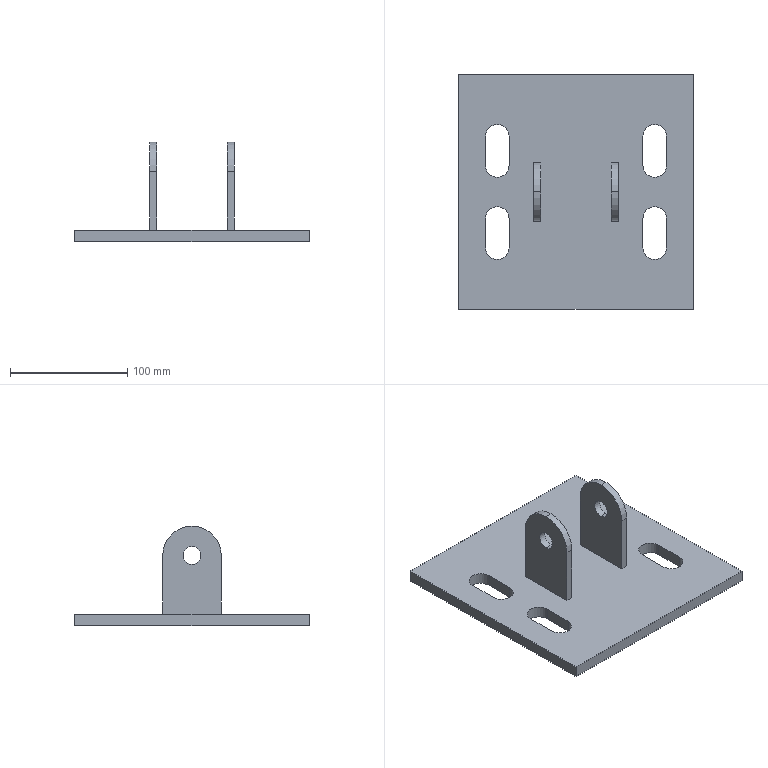Part | SolidWorks | features ICE 5, Extrusion 1 | 1 solid | 38 faces | box 200 x 200 x 85 mm | volume 407094 mm3 | plane 22 | cylinder 16 | commonest cylinder face diameters 20 x8 15 x4 50 x4
STEP:
#1=CARTESIAN_POINT('',(-30.,0.,47.5));
#2=VERTEX_POINT('',#1);
#3=CARTESIAN_POINT('',(-30.,0.,62.5));
#4=VERTEX_POINT('',#3);
#5=CARTESIAN_POINT('',(-30.,0.,55.));
#6=DIRECTION('',(-1.,0.,0.));
#7=DIRECTION('',(0.,0.,1.));
#8=AXIS2_PLACEMENT_3D('',#5,#6,#7);
#9=CIRCLE('',#8,7.5);
#10=EDGE_CURVE('',#2,#4,#9,.T.);
#11=ORIENTED_EDGE('',*,*,#10,.F.);
#12=CARTESIAN_POINT('',(-36.,0.,47.5));
#13=VERTEX_POINT('',#12);
#14=CARTESIAN_POINT('',(158.,0.,47.5));
#15=DIRECTION('',(-1.,0.,0.));
#16=VECTOR('',#15,1000.);
#17=LINE('',#14,#16);
#18=EDGE_CURVE('',#2,#13,#17,.T.);
#19=ORIENTED_EDGE('',*,*,#18,.T.);
#20=CARTESIAN_POINT('',(-36.,0.,62.5));
#21=VERTEX_POINT('',#20);
#22=CARTESIAN_POINT('',(-36.,0.,55.));
#23=DIRECTION('',(-1.,0.,0.));
#24=DIRECTION('',(0.,0.,1.));
#25=AXIS2_PLACEMENT_3D('',#22,#23,#24);
#26=CIRCLE('',#25,7.5);
#27=EDGE_CURVE('',#13,#21,#26,.T.);
#28=ORIENTED_EDGE('',*,*,#27,.T.);
#29=CARTESIAN_POINT('',(158.,0.,62.5));
#30=DIRECTION('',(-1.,0.,0.));
#31=VECTOR('',#30,1000.);
#32=LINE('',#29,#31);
#33=EDGE_CURVE('',#4,#21,#32,.T.);
#34=ORIENTED_EDGE('',*,*,#33,.F.);
#35=EDGE_LOOP('',(#11,#19,#28,#34));
#36=FACE_OUTER_BOUND('',#35,.T.);
#37=CARTESIAN_POINT('',(158.,0.,55.));
#38=DIRECTION('',(-1.,0.,0.));
#39=DIRECTION('',(0.,0.,1.));
#40=AXIS2_PLACEMENT_3D('',#37,#38,#39);
#41=CYLINDRICAL_SURFACE('',#40,7.5);
#42=ADVANCED_FACE('',(#36),#41,.F.);
#43=CARTESIAN_POINT('',(36.,0.,47.5));
#44=VERTEX_POINT('',#43);
#45=CARTESIAN_POINT('',(36.,0.,62.5));
#46=VERTEX_POINT('',#45);
#47=CARTESIAN_POINT('',(36.,0.,55.));
#48=DIRECTION('',(-1.,0.,0.));
#49=DIRECTION('',(0.,0.,1.));
#50=AXIS2_PLACEMENT_3D('',#47,#48,#49);
#51=CIRCLE('',#50,7.5);
#52=EDGE_CURVE('',#44,#46,#51,.T.);
#53=ORIENTED_EDGE('',*,*,#52,.F.);
#54=CARTESIAN_POINT('',(30.,0.,47.5));
#55=VERTEX_POINT('',#54);
#56=CARTESIAN_POINT('',(158.,0.,47.5));
#57=DIRECTION('',(-1.,0.,0.));
#58=VECTOR('',#57,1000.);
#59=LINE('',#56,#58);
#60=EDGE_CURVE('',#44,#55,#59,.T.);
#61=ORIENTED_EDGE('',*,*,#60,.T.);
#62=CARTESIAN_POINT('',(30.,0.,62.5));
#63=VERTEX_POINT('',#62);
#64=CARTESIAN_POINT('',(30.,0.,55.));
#65=DIRECTION('',(1.,0.,0.));
#66=DIRECTION('',(0.,0.,-1.));
#67=AXIS2_PLACEMENT_3D('',#64,#65,#66);
#68=CIRCLE('',#67,7.5);
#69=EDGE_CURVE('',#63,#55,#68,.T.);
#70=ORIENTED_EDGE('',*,*,#69,.F.);
#71=CARTESIAN_POINT('',(158.,0.,62.5));
#72=DIRECTION('',(-1.,0.,0.));
#73=VECTOR('',#72,1000.);
#74=LINE('',#71,#73);
#75=EDGE_CURVE('',#46,#63,#74,.T.);
#76=ORIENTED_EDGE('',*,*,#75,.F.);
#77=EDGE_LOOP('',(#53,#61,#70,#76));
#78=FACE_OUTER_BOUND('',#77,.T.);
#79=CARTESIAN_POINT('',(158.,0.,55.));
#80=DIRECTION('',(-1.,0.,0.));
#81=DIRECTION('',(0.,0.,1.));
#82=AXIS2_PLACEMENT_3D('',#79,#80,#81);
#83=CYLINDRICAL_SURFACE('',#82,7.5);
#84=ADVANCED_FACE('',(#78),#83,.F.);
#85=CARTESIAN_POINT('',(-30.,-25.,55.));
#86=VERTEX_POINT('',#85);
#87=CARTESIAN_POINT('',(-30.,0.,80.));
#88=VERTEX_POINT('',#87);
#89=CARTESIAN_POINT('',(-30.,0.,55.));
#90=DIRECTION('',(-1.,0.,0.));
#91=DIRECTION('',(0.,0.,1.));
#92=AXIS2_PLACEMENT_3D('',#89,#90,#91);
#93=CIRCLE('',#92,25.);
#94=EDGE_CURVE('',#86,#88,#93,.T.);
#95=ORIENTED_EDGE('',*,*,#94,.T.);
#96=CARTESIAN_POINT('',(-36.,0.,80.));
#97=VERTEX_POINT('',#96);
#98=CARTESIAN_POINT('',(-30.,0.,80.));
#99=DIRECTION('',(-1.,0.,0.));
#100=VECTOR('',#99,1000.);
#101=LINE('',#98,#100);
#102=EDGE_CURVE('',#88,#97,#101,.T.);
#103=ORIENTED_EDGE('',*,*,#102,.T.);
#104=CARTESIAN_POINT('',(-36.,-25.,55.));
#105=VERTEX_POINT('',#104);
#106=CARTESIAN_POINT('',(-36.,0.,55.));
#107=DIRECTION('',(-1.,0.,0.));
#108=DIRECTION('',(0.,0.,1.));
#109=AXIS2_PLACEMENT_3D('',#106,#107,#108);
#110=CIRCLE('',#109,25.);
#111=EDGE_CURVE('',#105,#97,#110,.T.);
#112=ORIENTED_EDGE('',*,*,#111,.F.);
#113=CARTESIAN_POINT('',(-36.,-25.,55.));
#114=DIRECTION('',(1.,0.,0.));
#115=VECTOR('',#114,1000.);
#116=LINE('',#113,#115);
#117=EDGE_CURVE('',#105,#86,#116,.T.);
#118=ORIENTED_EDGE('',*,*,#117,.T.);
#119=EDGE_LOOP('',(#95,#103,#112,#118));
#120=FACE_OUTER_BOUND('',#119,.T.);
#121=CARTESIAN_POINT('',(-30.,0.,55.));
#122=DIRECTION('',(-1.,0.,0.));
#123=DIRECTION('',(0.,0.,1.));
#124=AXIS2_PLACEMENT_3D('',#121,#122,#123);
#125=CYLINDRICAL_SURFACE('',#124,25.);
#126=ADVANCED_FACE('',(#120),#125,.T.);
#127=CARTESIAN_POINT('',(36.,-25.,55.));
#128=VERTEX_POINT('',#127);
#129=CARTESIAN_POINT('',(36.,0.,80.));
#130=VERTEX_POINT('',#129);
#131=CARTESIAN_POINT('',(36.,0.,55.));
#132=DIRECTION('',(-1.,0.,0.));
#133=DIRECTION('',(0.,0.,1.));
#134=AXIS2_PLACEMENT_3D('',#131,#132,#133);
#135=CIRCLE('',#134,25.);
#136=EDGE_CURVE('',#128,#130,#135,.T.);
#137=ORIENTED_EDGE('',*,*,#136,.T.);
#138=CARTESIAN_POINT('',(30.,0.,80.));
#139=VERTEX_POINT('',#138);
#140=CARTESIAN_POINT('',(36.,0.,80.));
#141=DIRECTION('',(-1.,0.,0.));
#142=VECTOR('',#141,1000.);
#143=LINE('',#140,#142);
#144=EDGE_CURVE('',#130,#139,#143,.T.);
#145=ORIENTED_EDGE('',*,*,#144,.T.);
#146=CARTESIAN_POINT('',(30.,-25.,55.));
#147=VERTEX_POINT('',#146);
#148=CARTESIAN_POINT('',(30.,0.,55.));
#149=DIRECTION('',(-1.,0.,0.));
#150=DIRECTION('',(0.,0.,1.));
#151=AXIS2_PLACEMENT_3D('',#148,#149,#150);
#152=CIRCLE('',#151,25.);
#153=EDGE_CURVE('',#147,#139,#152,.T.);
#154=ORIENTED_EDGE('',*,*,#153,.F.);
#155=CARTESIAN_POINT('',(36.,-25.,55.));
#156=DIRECTION('',(1.,0.,0.));
#157=VECTOR('',#156,1000.);
#158=LINE('',#155,#157);
#159=EDGE_CURVE('',#147,#128,#158,.T.);
#160=ORIENTED_EDGE('',*,*,#159,.T.);
#161=EDGE_LOOP('',(#137,#145,#154,#160));
#162=FACE_OUTER_BOUND('',#161,.T.);
#163=CARTESIAN_POINT('',(36.,0.,55.));
#164=DIRECTION('',(-1.,0.,0.));
#165=DIRECTION('',(0.,0.,1.));
#166=AXIS2_PLACEMENT_3D('',#163,#164,#165);
#167=CYLINDRICAL_SURFACE('',#166,25.);
#168=ADVANCED_FACE('',(#162),#167,.T.);
#169=CARTESIAN_POINT('',(57.064,47.5,5.));
#170=VERTEX_POINT('',#169);
#171=CARTESIAN_POINT('',(57.064,22.5,5.));
#172=VERTEX_POINT('',#171);
#173=CARTESIAN_POINT('',(57.064,47.5,5.));
#174=DIRECTION('',(0.,-1.,0.));
#175=VECTOR('',#174,1000.);
#176=LINE('',#173,#175);
#177=EDGE_CURVE('',#170,#172,#176,.T.);
#178=ORIENTED_EDGE('',*,*,#177,.F.);
#179=CARTESIAN_POINT('',(77.064,47.5,5.));
#180=VERTEX_POINT('',#179);
#181=CARTESIAN_POINT('',(67.064,47.5,5.));
#182=DIRECTION('',(0.,0.,1.));
#183=DIRECTION('',(-1.,0.,0.));
#184=AXIS2_PLACEMENT_3D('',#181,#182,#183);
#185=CIRCLE('',#184,10.);
#186=EDGE_CURVE('',#180,#170,#185,.T.);
#187=ORIENTED_EDGE('',*,*,#186,.F.);
#188=CARTESIAN_POINT('',(77.064,22.5,5.));
#189=VERTEX_POINT('',#188);
#190=CARTESIAN_POINT('',(77.064,47.5,5.));
#191=DIRECTION('',(0.,1.,0.));
#192=VECTOR('',#191,1000.);
#193=LINE('',#190,#192);
#194=EDGE_CURVE('',#189,#180,#193,.T.);
#195=ORIENTED_EDGE('',*,*,#194,.F.);
#196=CARTESIAN_POINT('',(67.064,22.5,5.));
#197=DIRECTION('',(0.,0.,1.));
#198=DIRECTION('',(-1.,0.,0.));
#199=AXIS2_PLACEMENT_3D('',#196,#197,#198);
#200=CIRCLE('',#199,10.);
#201=EDGE_CURVE('',#172,#189,#200,.T.);
#202=ORIENTED_EDGE('',*,*,#201,.F.);
#203=EDGE_LOOP('',(#178,#187,#195,#202));
#204=FACE_BOUND('',#203,.T.);
#205=CARTESIAN_POINT('',(57.064,-22.5,5.));
#206=VERTEX_POINT('',#205);
#207=CARTESIAN_POINT('',(57.064,-47.5,5.));
#208=VERTEX_POINT('',#207);
#209=CARTESIAN_POINT('',(57.064,-22.5,5.));
#210=DIRECTION('',(0.,-1.,0.));
#211=VECTOR('',#210,1000.);
#212=LINE('',#209,#211);
#213=EDGE_CURVE('',#206,#208,#212,.T.);
#214=ORIENTED_EDGE('',*,*,#213,.F.);
#215=CARTESIAN_POINT('',(77.064,-22.5,5.));
#216=VERTEX_POINT('',#215);
#217=CARTESIAN_POINT('',(67.064,-22.5,5.));
#218=DIRECTION('',(0.,0.,1.));
#219=DIRECTION('',(-1.,0.,0.));
#220=AXIS2_PLACEMENT_3D('',#217,#218,#219);
#221=CIRCLE('',#220,10.);
#222=EDGE_CURVE('',#216,#206,#221,.T.);
#223=ORIENTED_EDGE('',*,*,#222,.F.);
#224=CARTESIAN_POINT('',(77.064,-47.5,5.));
#225=VERTEX_POINT('',#224);
#226=CARTESIAN_POINT('',(77.064,-22.5,5.));
#227=DIRECTION('',(0.,1.,0.));
#228=VECTOR('',#227,1000.);
#229=LINE('',#226,#228);
#230=EDGE_CURVE('',#225,#216,#229,.T.);
#231=ORIENTED_EDGE('',*,*,#230,.F.);
#232=CARTESIAN_POINT('',(67.064,-47.5,5.));
#233=DIRECTION('',(0.,0.,1.));
#234=DIRECTION('',(-1.,0.,0.));
#235=AXIS2_PLACEMENT_3D('',#232,#233,#234);
#236=CIRCLE('',#235,10.);
#237=EDGE_CURVE('',#208,#225,#236,.T.);
#238=ORIENTED_EDGE('',*,*,#237,.F.);
#239=EDGE_LOOP('',(#214,#223,#231,#238));
#240=FACE_BOUND('',#239,.T.);
#241=CARTESIAN_POINT('',(-77.064,-22.5,5.));
#242=VERTEX_POINT('',#241);
#243=CARTESIAN_POINT('',(-77.064,-47.5,5.));
#244=VERTEX_POINT('',#243);
#245=CARTESIAN_POINT('',(-77.064,-22.5,5.));
#246=DIRECTION('',(0.,-1.,0.));
#247=VECTOR('',#246,1000.);
#248=LINE('',#245,#247);
#249=EDGE_CURVE('',#242,#244,#248,.T.);
#250=ORIENTED_EDGE('',*,*,#249,.F.);
#251=CARTESIAN_POINT('',(-57.064,-22.5,5.));
#252=VERTEX_POINT('',#251);
#253=CARTESIAN_POINT('',(-67.064,-22.5,5.));
#254=DIRECTION('',(0.,0.,1.));
#255=DIRECTION('',(1.,0.,0.));
#256=AXIS2_PLACEMENT_3D('',#253,#254,#255);
#257=CIRCLE('',#256,10.);
#258=EDGE_CURVE('',#252,#242,#257,.T.);
#259=ORIENTED_EDGE('',*,*,#258,.F.);
#260=CARTESIAN_POINT('',(-57.064,-47.5,5.));
#261=VERTEX_POINT('',#260);
#262=CARTESIAN_POINT('',(-57.064,-22.5,5.));
#263=DIRECTION('',(0.,1.,0.));
#264=VECTOR('',#263,1000.);
#265=LINE('',#262,#264);
#266=EDGE_CURVE('',#261,#252,#265,.T.);
#267=ORIENTED_EDGE('',*,*,#266,.F.);
#268=CARTESIAN_POINT('',(-67.064,-47.5,5.));
#269=DIRECTION('',(0.,0.,1.));
#270=DIRECTION('',(1.,0.,0.));
#271=AXIS2_PLACEMENT_3D('',#268,#269,#270);
#272=CIRCLE('',#271,10.);
#273=EDGE_CURVE('',#244,#261,#272,.T.);
#274=ORIENTED_EDGE('',*,*,#273,.F.);
#275=EDGE_LOOP('',(#250,#259,#267,#274));
#276=FACE_BOUND('',#275,.T.);
#277=CARTESIAN_POINT('',(-77.064,47.5,5.));
#278=VERTEX_POINT('',#277);
#279=CARTESIAN_POINT('',(-77.064,22.5,5.));
#280=VERTEX_POINT('',#279);
#281=CARTESIAN_POINT('',(-77.064,47.5,5.));
#282=DIRECTION('',(0.,-1.,0.));
#283=VECTOR('',#282,1000.);
#284=LINE('',#281,#283);
#285=EDGE_CURVE('',#278,#280,#284,.T.);
#286=ORIENTED_EDGE('',*,*,#285,.F.);
#287=CARTESIAN_POINT('',(-57.064,47.5,5.));
#288=VERTEX_POINT('',#287);
#289=CARTESIAN_POINT('',(-67.064,47.5,5.));
#290=DIRECTION('',(0.,0.,1.));
#291=DIRECTION('',(1.,0.,0.));
#292=AXIS2_PLACEMENT_3D('',#289,#290,#291);
#293=CIRCLE('',#292,10.);
#294=EDGE_CURVE('',#288,#278,#293,.T.);
#295=ORIENTED_EDGE('',*,*,#294,.F.);
#296=CARTESIAN_POINT('',(-57.064,22.5,5.));
#297=VERTEX_POINT('',#296);
#298=CARTESIAN_POINT('',(-57.064,47.5,5.));
#299=DIRECTION('',(0.,1.,0.));
#300=VECTOR('',#299,1000.);
#301=LINE('',#298,#300);
#302=EDGE_CURVE('',#297,#288,#301,.T.);
#303=ORIENTED_EDGE('',*,*,#302,.F.);
#304=CARTESIAN_POINT('',(-67.064,22.5,5.));
#305=DIRECTION('',(0.,0.,1.));
#306=DIRECTION('',(1.,0.,0.));
#307=AXIS2_PLACEMENT_3D('',#304,#305,#306);
#308=CIRCLE('',#307,10.);
#309=EDGE_CURVE('',#280,#297,#308,.T.);
#310=ORIENTED_EDGE('',*,*,#309,.F.);
#311=EDGE_LOOP('',(#286,#295,#303,#310));
#312=FACE_BOUND('',#311,.T.);
#313=CARTESIAN_POINT('',(-30.,-25.,5.));
#314=VERTEX_POINT('',#313);
#315=CARTESIAN_POINT('',(-30.,25.,5.));
#316=VERTEX_POINT('',#315);
#317=CARTESIAN_POINT('',(-30.,-25.,5.));
#318=DIRECTION('',(0.,1.,0.));
#319=VECTOR('',#318,1000.);
#320=LINE('',#317,#319);
#321=EDGE_CURVE('',#314,#316,#320,.T.);
#322=ORIENTED_EDGE('',*,*,#321,.F.);
#323=CARTESIAN_POINT('',(-36.,-25.,5.));
#324=VERTEX_POINT('',#323);
#325=CARTESIAN_POINT('',(-36.,-25.,5.));
#326=DIRECTION('',(1.,0.,0.));
#327=VECTOR('',#326,1000.);
#328=LINE('',#325,#327);
#329=EDGE_CURVE('',#324,#314,#328,.T.);
#330=ORIENTED_EDGE('',*,*,#329,.F.);
#331=CARTESIAN_POINT('',(-36.,25.,5.));
#332=VERTEX_POINT('',#331);
#333=CARTESIAN_POINT('',(-36.,-25.,5.));
#334=DIRECTION('',(0.,-1.,0.));
#335=VECTOR('',#334,1000.);
#336=LINE('',#333,#335);
#337=EDGE_CURVE('',#332,#324,#336,.T.);
#338=ORIENTED_EDGE('',*,*,#337,.F.);
#339=CARTESIAN_POINT('',(-36.,25.,5.));
#340=DIRECTION('',(-1.,0.,0.));
#341=VECTOR('',#340,1000.);
#342=LINE('',#339,#341);
#343=EDGE_CURVE('',#316,#332,#342,.T.);
#344=ORIENTED_EDGE('',*,*,#343,.F.);
#345=EDGE_LOOP('',(#322,#330,#338,#344));
#346=FACE_BOUND('',#345,.T.);
#347=CARTESIAN_POINT('',(-100.,100.,5.));
#348=VERTEX_POINT('',#347);
#349=CARTESIAN_POINT('',(-100.,-100.,5.));
#350=VERTEX_POINT('',#349);
#351=CARTESIAN_POINT('',(-100.,100.,5.));
#352=DIRECTION('',(0.,-1.,0.));
#353=VECTOR('',#352,1000.);
#354=LINE('',#351,#353);
#355=EDGE_CURVE('',#348,#350,#354,.T.);
#356=ORIENTED_EDGE('',*,*,#355,.T.);
#357=CARTESIAN_POINT('',(100.,-100.,5.));
#358=VERTEX_POINT('',#357);
#359=CARTESIAN_POINT('',(100.,-100.,5.));
#360=DIRECTION('',(1.,0.,0.));
#361=VECTOR('',#360,1000.);
#362=LINE('',#359,#361);
#363=EDGE_CURVE('',#350,#358,#362,.T.);
#364=ORIENTED_EDGE('',*,*,#363,.T.);
#365=CARTESIAN_POINT('',(100.,100.,5.));
#366=VERTEX_POINT('',#365);
#367=CARTESIAN_POINT('',(100.,100.,5.));
#368=DIRECTION('',(0.,1.,0.));
#369=VECTOR('',#368,1000.);
#370=LINE('',#367,#369);
#371=EDGE_CURVE('',#358,#366,#370,.T.);
#372=ORIENTED_EDGE('',*,*,#371,.T.);
#373=CARTESIAN_POINT('',(100.,100.,5.));
#374=DIRECTION('',(-1.,0.,0.));
#375=VECTOR('',#374,1000.);
#376=LINE('',#373,#375);
#377=EDGE_CURVE('',#366,#348,#376,.T.);
#378=ORIENTED_EDGE('',*,*,#377,.T.);
#379=EDGE_LOOP('',(#356,#364,#372,#378));
#380=FACE_OUTER_BOUND('',#379,.T.);
#381=CARTESIAN_POINT('',(36.,-25.,5.));
#382=VERTEX_POINT('',#381);
#383=CARTESIAN_POINT('',(36.,25.,5.));
#384=VERTEX_POINT('',#383);
#385=CARTESIAN_POINT('',(36.,-25.,5.));
#386=DIRECTION('',(0.,1.,0.));
#387=VECTOR('',#386,1000.);
#388=LINE('',#385,#387);
#389=EDGE_CURVE('',#382,#384,#388,.T.);
#390=ORIENTED_EDGE('',*,*,#389,.F.);
#391=CARTESIAN_POINT('',(30.,-25.,5.));
#392=VERTEX_POINT('',#391);
#393=CARTESIAN_POINT('',(36.,-25.,5.));
#394=DIRECTION('',(1.,0.,0.));
#395=VECTOR('',#394,1000.);
#396=LINE('',#393,#395);
#397=EDGE_CURVE('',#392,#382,#396,.T.);
#398=ORIENTED_EDGE('',*,*,#397,.F.);
#399=CARTESIAN_POINT('',(30.,25.,5.));
#400=VERTEX_POINT('',#399);
#401=CARTESIAN_POINT('',(30.,-25.,5.));
#402=DIRECTION('',(0.,-1.,0.));
#403=VECTOR('',#402,1000.);
#404=LINE('',#401,#403);
#405=EDGE_CURVE('',#400,#392,#404,.T.);
#406=ORIENTED_EDGE('',*,*,#405,.F.);
#407=CARTESIAN_POINT('',(36.,25.,5.));
#408=DIRECTION('',(-1.,0.,0.));
#409=VECTOR('',#408,1000.);
#410=LINE('',#407,#409);
#411=EDGE_CURVE('',#384,#400,#410,.T.);
#412=ORIENTED_EDGE('',*,*,#411,.F.);
#413=EDGE_LOOP('',(#390,#398,#406,#412));
#414=FACE_BOUND('',#413,.T.);
#415=CARTESIAN_POINT('',(0.,0.,5.));
#416=DIRECTION('',(0.,0.,-1.));
#417=DIRECTION('',(-1.,0.,0.));
#418=AXIS2_PLACEMENT_3D('',#415,#416,#417);
#419=PLANE('',#418);
#420=ADVANCED_FACE('',(#204,#240,#276,#312,#346,#380,#414),#419,.F.);
#421=CARTESIAN_POINT('',(-100.,-100.,-5.));
#422=VERTEX_POINT('',#421);
#423=CARTESIAN_POINT('',(-100.,-100.,-5.));
#424=DIRECTION('',(0.,0.,1.));
#425=VECTOR('',#424,1000.);
#426=LINE('',#423,#425);
#427=EDGE_CURVE('',#422,#350,#426,.T.);
#428=ORIENTED_EDGE('',*,*,#427,.T.);
#429=ORIENTED_EDGE('',*,*,#355,.F.);
#430=CARTESIAN_POINT('',(-100.,100.,-5.));
#431=VERTEX_POINT('',#430);
#432=CARTESIAN_POINT('',(-100.,100.,-5.));
#433=DIRECTION('',(0.,0.,1.));
#434=VECTOR('',#433,1000.);
#435=LINE('',#432,#434);
#436=EDGE_CURVE('',#431,#348,#435,.T.);
#437=ORIENTED_EDGE('',*,*,#436,.F.);
#438=CARTESIAN_POINT('',(-100.,100.,-5.));
#439=DIRECTION('',(0.,-1.,0.));
#440=VECTOR('',#439,1000.);
#441=LINE('',#438,#440);
#442=EDGE_CURVE('',#431,#422,#441,.T.);
#443=ORIENTED_EDGE('',*,*,#442,.T.);
#444=EDGE_LOOP('',(#428,#429,#437,#443));
#445=FACE_OUTER_BOUND('',#444,.T.);
#446=CARTESIAN_POINT('',(-100.,100.,-5.));
#447=DIRECTION('',(-1.,0.,0.));
#448=DIRECTION('',(0.,-1.,0.));
#449=AXIS2_PLACEMENT_3D('',#446,#447,#448);
#450=PLANE('',#449);
#451=ADVANCED_FACE('',(#445),#450,.T.);
#452=ORIENTED_EDGE('',*,*,#436,.T.);
#453=ORIENTED_EDGE('',*,*,#377,.F.);
#454=CARTESIAN_POINT('',(100.,100.,-5.));
#455=VERTEX_POINT('',#454);
#456=CARTESIAN_POINT('',(100.,100.,-5.));
#457=DIRECTION('',(0.,0.,1.));
#458=VECTOR('',#457,1000.);
#459=LINE('',#456,#458);
#460=EDGE_CURVE('',#455,#366,#459,.T.);
#461=ORIENTED_EDGE('',*,*,#460,.F.);
#462=CARTESIAN_POINT('',(100.,100.,-5.));
#463=DIRECTION('',(-1.,0.,0.));
#464=VECTOR('',#463,1000.);
#465=LINE('',#462,#464);
#466=EDGE_CURVE('',#455,#431,#465,.T.);
#467=ORIENTED_EDGE('',*,*,#466,.T.);
#468=EDGE_LOOP('',(#452,#453,#461,#467));
#469=FACE_OUTER_BOUND('',#468,.T.);
#470=CARTESIAN_POINT('',(100.,100.,-5.));
#471=DIRECTION('',(0.,1.,0.));
#472=DIRECTION('',(-1.,0.,0.));
#473=AXIS2_PLACEMENT_3D('',#470,#471,#472);
#474=PLANE('',#473);
#475=ADVANCED_FACE('',(#469),#474,.T.);
#476=ORIENTED_EDGE('',*,*,#460,.T.);
#477=ORIENTED_EDGE('',*,*,#371,.F.);
#478=CARTESIAN_POINT('',(100.,-100.,-5.));
#479=VERTEX_POINT('',#478);
#480=CARTESIAN_POINT('',(100.,-100.,-5.));
#481=DIRECTION('',(0.,0.,1.));
#482=VECTOR('',#481,1000.);
#483=LINE('',#480,#482);
#484=EDGE_CURVE('',#479,#358,#483,.T.);
#485=ORIENTED_EDGE('',*,*,#484,.F.);
#486=CARTESIAN_POINT('',(100.,100.,-5.));
#487=DIRECTION('',(0.,1.,0.));
#488=VECTOR('',#487,1000.);
#489=LINE('',#486,#488);
#490=EDGE_CURVE('',#479,#455,#489,.T.);
#491=ORIENTED_EDGE('',*,*,#490,.T.);
#492=EDGE_LOOP('',(#476,#477,#485,#491));
#493=FACE_OUTER_BOUND('',#492,.T.);
#494=CARTESIAN_POINT('',(100.,100.,-5.));
#495=DIRECTION('',(1.,0.,0.));
#496=DIRECTION('',(0.,1.,0.));
#497=AXIS2_PLACEMENT_3D('',#494,#495,#496);
#498=PLANE('',#497);
#499=ADVANCED_FACE('',(#493),#498,.T.);
#500=ORIENTED_EDGE('',*,*,#484,.T.);
#501=ORIENTED_EDGE('',*,*,#363,.F.);
#502=ORIENTED_EDGE('',*,*,#427,.F.);
#503=CARTESIAN_POINT('',(100.,-100.,-5.));
#504=DIRECTION('',(1.,0.,0.));
#505=VECTOR('',#504,1000.);
#506=LINE('',#503,#505);
#507=EDGE_CURVE('',#422,#479,#506,.T.);
#508=ORIENTED_EDGE('',*,*,#507,.T.);
#509=EDGE_LOOP('',(#500,#501,#502,#508));
#510=FACE_OUTER_BOUND('',#509,.T.);
#511=CARTESIAN_POINT('',(100.,-100.,-5.));
#512=DIRECTION('',(0.,-1.,0.));
#513=DIRECTION('',(1.,0.,0.));
#514=AXIS2_PLACEMENT_3D('',#511,#512,#513);
#515=PLANE('',#514);
#516=ADVANCED_FACE('',(#510),#515,.T.);
#517=CARTESIAN_POINT('',(77.064,47.5,-5.));
#518=VERTEX_POINT('',#517);
#519=CARTESIAN_POINT('',(57.064,47.5,-5.));
#520=VERTEX_POINT('',#519);
#521=CARTESIAN_POINT('',(67.064,47.5,-5.));
#522=DIRECTION('',(0.,0.,1.));
#523=DIRECTION('',(-1.,0.,0.));
#524=AXIS2_PLACEMENT_3D('',#521,#522,#523);
#525=CIRCLE('',#524,10.);
#526=EDGE_CURVE('',#518,#520,#525,.T.);
#527=ORIENTED_EDGE('',*,*,#526,.T.);
#528=CARTESIAN_POINT('',(57.064,22.5,-5.));
#529=VERTEX_POINT('',#528);
#530=CARTESIAN_POINT('',(57.064,47.5,-5.));
#531=DIRECTION('',(0.,-1.,0.));
#532=VECTOR('',#531,1000.);
#533=LINE('',#530,#532);
#534=EDGE_CURVE('',#520,#529,#533,.T.);
#535=ORIENTED_EDGE('',*,*,#534,.T.);
#536=CARTESIAN_POINT('',(77.064,22.5,-5.));
#537=VERTEX_POINT('',#536);
#538=CARTESIAN_POINT('',(67.064,22.5,-5.));
#539=DIRECTION('',(0.,0.,1.));
#540=DIRECTION('',(-1.,0.,0.));
#541=AXIS2_PLACEMENT_3D('',#538,#539,#540);
#542=CIRCLE('',#541,10.);
#543=EDGE_CURVE('',#529,#537,#542,.T.);
#544=ORIENTED_EDGE('',*,*,#543,.T.);
#545=CARTESIAN_POINT('',(77.064,47.5,-5.));
#546=DIRECTION('',(0.,1.,0.));
#547=VECTOR('',#546,1000.);
#548=LINE('',#545,#547);
#549=EDGE_CURVE('',#537,#518,#548,.T.);
#550=ORIENTED_EDGE('',*,*,#549,.T.);
#551=EDGE_LOOP('',(#527,#535,#544,#550));
#552=FACE_BOUND('',#551,.T.);
#553=CARTESIAN_POINT('',(77.064,-22.5,-5.));
#554=VERTEX_POINT('',#553);
#555=CARTESIAN_POINT('',(57.064,-22.5,-5.));
#556=VERTEX_POINT('',#555);
#557=CARTESIAN_POINT('',(67.064,-22.5,-5.));
#558=DIRECTION('',(0.,0.,1.));
#559=DIRECTION('',(-1.,0.,0.));
#560=AXIS2_PLACEMENT_3D('',#557,#558,#559);
#561=CIRCLE('',#560,10.);
#562=EDGE_CURVE('',#554,#556,#561,.T.);
#563=ORIENTED_EDGE('',*,*,#562,.T.);
#564=CARTESIAN_POINT('',(57.064,-47.5,-5.));
#565=VERTEX_POINT('',#564);
#566=CARTESIAN_POINT('',(57.064,-22.5,-5.));
#567=DIRECTION('',(0.,-1.,0.));
#568=VECTOR('',#567,1000.);
#569=LINE('',#566,#568);
#570=EDGE_CURVE('',#556,#565,#569,.T.);
#571=ORIENTED_EDGE('',*,*,#570,.T.);
#572=CARTESIAN_POINT('',(77.064,-47.5,-5.));
#573=VERTEX_POINT('',#572);
#574=CARTESIAN_POINT('',(67.064,-47.5,-5.));
#575=DIRECTION('',(0.,0.,1.));
#576=DIRECTION('',(-1.,0.,0.));
#577=AXIS2_PLACEMENT_3D('',#574,#575,#576);
#578=CIRCLE('',#577,10.);
#579=EDGE_CURVE('',#565,#573,#578,.T.);
#580=ORIENTED_EDGE('',*,*,#579,.T.);
#581=CARTESIAN_POINT('',(77.064,-22.5,-5.));
#582=DIRECTION('',(0.,1.,0.));
#583=VECTOR('',#582,1000.);
#584=LINE('',#581,#583);
#585=EDGE_CURVE('',#573,#554,#584,.T.);
#586=ORIENTED_EDGE('',*,*,#585,.T.);
#587=EDGE_LOOP('',(#563,#571,#580,#586));
#588=FACE_BOUND('',#587,.T.);
#589=CARTESIAN_POINT('',(-57.064,-22.5,-5.));
#590=VERTEX_POINT('',#589);
#591=CARTESIAN_POINT('',(-77.064,-22.5,-5.));
#592=VERTEX_POINT('',#591);
#593=CARTESIAN_POINT('',(-67.064,-22.5,-5.));
#594=DIRECTION('',(0.,0.,1.));
#595=DIRECTION('',(1.,0.,0.));
#596=AXIS2_PLACEMENT_3D('',#593,#594,#595);
#597=CIRCLE('',#596,10.);
#598=EDGE_CURVE('',#590,#592,#597,.T.);
#599=ORIENTED_EDGE('',*,*,#598,.T.);
#600=CARTESIAN_POINT('',(-77.064,-47.5,-5.));
#601=VERTEX_POINT('',#600);
#602=CARTESIAN_POINT('',(-77.064,-22.5,-5.));
#603=DIRECTION('',(0.,-1.,0.));
#604=VECTOR('',#603,1000.);
#605=LINE('',#602,#604);
#606=EDGE_CURVE('',#592,#601,#605,.T.);
#607=ORIENTED_EDGE('',*,*,#606,.T.);
#608=CARTESIAN_POINT('',(-57.064,-47.5,-5.));
#609=VERTEX_POINT('',#608);
#610=CARTESIAN_POINT('',(-67.064,-47.5,-5.));
#611=DIRECTION('',(0.,0.,1.));
#612=DIRECTION('',(1.,0.,0.));
#613=AXIS2_PLACEMENT_3D('',#610,#611,#612);
#614=CIRCLE('',#613,10.);
#615=EDGE_CURVE('',#601,#609,#614,.T.);
#616=ORIENTED_EDGE('',*,*,#615,.T.);
#617=CARTESIAN_POINT('',(-57.064,-22.5,-5.));
#618=DIRECTION('',(0.,1.,0.));
#619=VECTOR('',#618,1000.);
#620=LINE('',#617,#619);
#621=EDGE_CURVE('',#609,#590,#620,.T.);
#622=ORIENTED_EDGE('',*,*,#621,.T.);
#623=EDGE_LOOP('',(#599,#607,#616,#622));
#624=FACE_BOUND('',#623,.T.);
#625=CARTESIAN_POINT('',(-57.064,47.5,-5.));
#626=VERTEX_POINT('',#625);
#627=CARTESIAN_POINT('',(-77.064,47.5,-5.));
#628=VERTEX_POINT('',#627);
#629=CARTESIAN_POINT('',(-67.064,47.5,-5.));
#630=DIRECTION('',(0.,0.,1.));
#631=DIRECTION('',(1.,0.,0.));
#632=AXIS2_PLACEMENT_3D('',#629,#630,#631);
#633=CIRCLE('',#632,10.);
#634=EDGE_CURVE('',#626,#628,#633,.T.);
#635=ORIENTED_EDGE('',*,*,#634,.T.);
#636=CARTESIAN_POINT('',(-77.064,22.5,-5.));
#637=VERTEX_POINT('',#636);
#638=CARTESIAN_POINT('',(-77.064,47.5,-5.));
#639=DIRECTION('',(0.,-1.,0.));
#640=VECTOR('',#639,1000.);
#641=LINE('',#638,#640);
#642=EDGE_CURVE('',#628,#637,#641,.T.);
#643=ORIENTED_EDGE('',*,*,#642,.T.);
#644=CARTESIAN_POINT('',(-57.064,22.5,-5.));
#645=VERTEX_POINT('',#644);
#646=CARTESIAN_POINT('',(-67.064,22.5,-5.));
#647=DIRECTION('',(0.,0.,1.));
#648=DIRECTION('',(1.,0.,0.));
#649=AXIS2_PLACEMENT_3D('',#646,#647,#648);
#650=CIRCLE('',#649,10.);
#651=EDGE_CURVE('',#637,#645,#650,.T.);
#652=ORIENTED_EDGE('',*,*,#651,.T.);
#653=CARTESIAN_POINT('',(-57.064,47.5,-5.));
#654=DIRECTION('',(0.,1.,0.));
#655=VECTOR('',#654,1000.);
#656=LINE('',#653,#655);
#657=EDGE_CURVE('',#645,#626,#656,.T.);
#658=ORIENTED_EDGE('',*,*,#657,.T.);
#659=EDGE_LOOP('',(#635,#643,#652,#658));
#660=FACE_BOUND('',#659,.T.);
#661=ORIENTED_EDGE('',*,*,#442,.F.);
#662=ORIENTED_EDGE('',*,*,#466,.F.);
#663=ORIENTED_EDGE('',*,*,#490,.F.);
#664=ORIENTED_EDGE('',*,*,#507,.F.);
#665=EDGE_LOOP('',(#661,#662,#663,#664));
#666=FACE_OUTER_BOUND('',#665,.T.);
#667=CARTESIAN_POINT('',(0.,0.,-5.));
#668=DIRECTION('',(0.,0.,-1.));
#669=DIRECTION('',(-1.,0.,0.));
#670=AXIS2_PLACEMENT_3D('',#667,#668,#669);
#671=PLANE('',#670);
#672=ADVANCED_FACE('',(#552,#588,#624,#660,#666),#671,.T.);
#673=CARTESIAN_POINT('',(-30.,0.,55.));
#674=DIRECTION('',(-1.,0.,0.));
#675=DIRECTION('',(0.,0.,1.));
#676=AXIS2_PLACEMENT_3D('',#673,#674,#675);
#677=CIRCLE('',#676,7.5);
#678=EDGE_CURVE('',#4,#2,#677,.T.);
#679=ORIENTED_EDGE('',*,*,#678,.T.);
#680=ORIENTED_EDGE('',*,*,#10,.T.);
#681=EDGE_LOOP('',(#679,#680));
#682=FACE_BOUND('',#681,.T.);
#683=ORIENTED_EDGE('',*,*,#321,.T.);
#684=CARTESIAN_POINT('',(-30.,25.,55.));
#685=VERTEX_POINT('',#684);
#686=CARTESIAN_POINT('',(-30.,25.,55.));
#687=DIRECTION('',(0.,0.,-1.));
#688=VECTOR('',#687,1000.);
#689=LINE('',#686,#688);
#690=EDGE_CURVE('',#685,#316,#689,.T.);
#691=ORIENTED_EDGE('',*,*,#690,.F.);
#692=CARTESIAN_POINT('',(-30.,0.,55.));
#693=DIRECTION('',(-1.,0.,0.));
#694=DIRECTION('',(0.,0.,1.));
#695=AXIS2_PLACEMENT_3D('',#692,#693,#694);
#696=CIRCLE('',#695,25.);
#697=EDGE_CURVE('',#88,#685,#696,.T.);
#698=ORIENTED_EDGE('',*,*,#697,.F.);
#699=ORIENTED_EDGE('',*,*,#94,.F.);
#700=CARTESIAN_POINT('',(-30.,-25.,55.));
#701=DIRECTION('',(0.,0.,-1.));
#702=VECTOR('',#701,1000.);
#703=LINE('',#700,#702);
#704=EDGE_CURVE('',#86,#314,#703,.T.);
#705=ORIENTED_EDGE('',*,*,#704,.T.);
#706=EDGE_LOOP('',(#683,#691,#698,#699,#705));
#707=FACE_OUTER_BOUND('',#706,.T.);
#708=CARTESIAN_POINT('',(-30.,-25.,55.));
#709=DIRECTION('',(-1.,0.,0.));
#710=DIRECTION('',(0.,0.,1.));
#711=AXIS2_PLACEMENT_3D('',#708,#709,#710);
#712=PLANE('',#711);
#713=ADVANCED_FACE('',(#682,#707),#712,.F.);
#714=ORIENTED_EDGE('',*,*,#343,.T.);
#715=CARTESIAN_POINT('',(-36.,25.,55.));
#716=VERTEX_POINT('',#715);
#717=CARTESIAN_POINT('',(-36.,25.,55.));
#718=DIRECTION('',(0.,0.,-1.));
#719=VECTOR('',#718,1000.);
#720=LINE('',#717,#719);
#721=EDGE_CURVE('',#716,#332,#720,.T.);
#722=ORIENTED_EDGE('',*,*,#721,.F.);
#723=CARTESIAN_POINT('',(-36.,25.,55.));
#724=DIRECTION('',(-1.,0.,0.));
#725=VECTOR('',#724,1000.);
#726=LINE('',#723,#725);
#727=EDGE_CURVE('',#685,#716,#726,.T.);
#728=ORIENTED_EDGE('',*,*,#727,.F.);
#729=ORIENTED_EDGE('',*,*,#690,.T.);
#730=EDGE_LOOP('',(#714,#722,#728,#729));
#731=FACE_OUTER_BOUND('',#730,.T.);
#732=CARTESIAN_POINT('',(-36.,25.,55.));
#733=DIRECTION('',(0.,-1.,0.));
#734=DIRECTION('',(0.,0.,-1.));
#735=AXIS2_PLACEMENT_3D('',#732,#733,#734);
#736=PLANE('',#735);
#737=ADVANCED_FACE('',(#731),#736,.F.);
#738=CARTESIAN_POINT('',(-36.,0.,55.));
#739=DIRECTION('',(-1.,0.,0.));
#740=DIRECTION('',(0.,0.,1.));
#741=AXIS2_PLACEMENT_3D('',#738,#739,#740);
#742=CIRCLE('',#741,7.5);
#743=EDGE_CURVE('',#21,#13,#742,.T.);
#744=ORIENTED_EDGE('',*,*,#743,.F.);
#745=ORIENTED_EDGE('',*,*,#27,.F.);
#746=EDGE_LOOP('',(#744,#745));
#747=FACE_BOUND('',#746,.T.);
#748=ORIENTED_EDGE('',*,*,#337,.T.);
#749=CARTESIAN_POINT('',(-36.,-25.,55.));
#750=DIRECTION('',(0.,0.,-1.));
#751=VECTOR('',#750,1000.);
#752=LINE('',#749,#751);
#753=EDGE_CURVE('',#105,#324,#752,.T.);
#754=ORIENTED_EDGE('',*,*,#753,.F.);
#755=ORIENTED_EDGE('',*,*,#111,.T.);
#756=CARTESIAN_POINT('',(-36.,0.,55.));
#757=DIRECTION('',(-1.,0.,0.));
#758=DIRECTION('',(0.,0.,1.));
#759=AXIS2_PLACEMENT_3D('',#756,#757,#758);
#760=CIRCLE('',#759,25.);
#761=EDGE_CURVE('',#97,#716,#760,.T.);
#762=ORIENTED_EDGE('',*,*,#761,.T.);
#763=ORIENTED_EDGE('',*,*,#721,.T.);
#764=EDGE_LOOP('',(#748,#754,#755,#762,#763));
#765=FACE_OUTER_BOUND('',#764,.T.);
#766=CARTESIAN_POINT('',(-36.,-25.,55.));
#767=DIRECTION('',(1.,0.,0.));
#768=DIRECTION('',(0.,0.,-1.));
#769=AXIS2_PLACEMENT_3D('',#766,#767,#768);
#770=PLANE('',#769);
#771=ADVANCED_FACE('',(#747,#765),#770,.F.);
#772=ORIENTED_EDGE('',*,*,#329,.T.);
#773=ORIENTED_EDGE('',*,*,#704,.F.);
#774=ORIENTED_EDGE('',*,*,#117,.F.);
#775=ORIENTED_EDGE('',*,*,#753,.T.);
#776=EDGE_LOOP('',(#772,#773,#774,#775));
#777=FACE_OUTER_BOUND('',#776,.T.);
#778=CARTESIAN_POINT('',(-36.,-25.,55.));
#779=DIRECTION('',(0.,1.,0.));
#780=DIRECTION('',(0.,0.,1.));
#781=AXIS2_PLACEMENT_3D('',#778,#779,#780);
#782=PLANE('',#781);
#783=ADVANCED_FACE('',(#777),#782,.F.);
#784=CARTESIAN_POINT('',(36.,0.,55.));
#785=DIRECTION('',(-1.,0.,0.));
#786=DIRECTION('',(0.,0.,1.));
#787=AXIS2_PLACEMENT_3D('',#784,#785,#786);
#788=CIRCLE('',#787,7.5);
#789=EDGE_CURVE('',#46,#44,#788,.T.);
#790=ORIENTED_EDGE('',*,*,#789,.T.);
#791=ORIENTED_EDGE('',*,*,#52,.T.);
#792=EDGE_LOOP('',(#790,#791));
#793=FACE_BOUND('',#792,.T.);
#794=ORIENTED_EDGE('',*,*,#389,.T.);
#795=CARTESIAN_POINT('',(36.,25.,55.));
#796=VERTEX_POINT('',#795);
#797=CARTESIAN_POINT('',(36.,25.,55.));
#798=DIRECTION('',(0.,0.,-1.));
#799=VECTOR('',#798,1000.);
#800=LINE('',#797,#799);
#801=EDGE_CURVE('',#796,#384,#800,.T.);
#802=ORIENTED_EDGE('',*,*,#801,.F.);
#803=CARTESIAN_POINT('',(36.,0.,55.));
#804=DIRECTION('',(-1.,0.,0.));
#805=DIRECTION('',(0.,0.,1.));
#806=AXIS2_PLACEMENT_3D('',#803,#804,#805);
#807=CIRCLE('',#806,25.);
#808=EDGE_CURVE('',#130,#796,#807,.T.);
#809=ORIENTED_EDGE('',*,*,#808,.F.);
#810=ORIENTED_EDGE('',*,*,#136,.F.);
#811=CARTESIAN_POINT('',(36.,-25.,55.));
#812=DIRECTION('',(0.,0.,-1.));
#813=VECTOR('',#812,1000.);
#814=LINE('',#811,#813);
#815=EDGE_CURVE('',#128,#382,#814,.T.);
#816=ORIENTED_EDGE('',*,*,#815,.T.);
#817=EDGE_LOOP('',(#794,#802,#809,#810,#816));
#818=FACE_OUTER_BOUND('',#817,.T.);
#819=CARTESIAN_POINT('',(36.,-25.,55.));
#820=DIRECTION('',(-1.,0.,0.));
#821=DIRECTION('',(0.,0.,1.));
#822=AXIS2_PLACEMENT_3D('',#819,#820,#821);
#823=PLANE('',#822);
#824=ADVANCED_FACE('',(#793,#818),#823,.F.);
#825=ORIENTED_EDGE('',*,*,#411,.T.);
#826=CARTESIAN_POINT('',(30.,25.,55.));
#827=VERTEX_POINT('',#826);
#828=CARTESIAN_POINT('',(30.,25.,55.));
#829=DIRECTION('',(0.,0.,-1.));
#830=VECTOR('',#829,1000.);
#831=LINE('',#828,#830);
#832=EDGE_CURVE('',#827,#400,#831,.T.);
#833=ORIENTED_EDGE('',*,*,#832,.F.);
#834=CARTESIAN_POINT('',(36.,25.,55.));
#835=DIRECTION('',(-1.,0.,0.));
#836=VECTOR('',#835,1000.);
#837=LINE('',#834,#836);
#838=EDGE_CURVE('',#796,#827,#837,.T.);
#839=ORIENTED_EDGE('',*,*,#838,.F.);
#840=ORIENTED_EDGE('',*,*,#801,.T.);
#841=EDGE_LOOP('',(#825,#833,#839,#840));
#842=FACE_OUTER_BOUND('',#841,.T.);
#843=CARTESIAN_POINT('',(36.,25.,55.));
#844=DIRECTION('',(0.,-1.,0.));
#845=DIRECTION('',(0.,0.,-1.));
#846=AXIS2_PLACEMENT_3D('',#843,#844,#845);
#847=PLANE('',#846);
#848=ADVANCED_FACE('',(#842),#847,.F.);
#849=ORIENTED_EDGE('',*,*,#69,.T.);
#850=CARTESIAN_POINT('',(30.,0.,55.));
#851=DIRECTION('',(1.,0.,0.));
#852=DIRECTION('',(0.,0.,-1.));
#853=AXIS2_PLACEMENT_3D('',#850,#851,#852);
#854=CIRCLE('',#853,7.5);
#855=EDGE_CURVE('',#55,#63,#854,.T.);
#856=ORIENTED_EDGE('',*,*,#855,.T.);
#857=EDGE_LOOP('',(#849,#856));
#858=FACE_BOUND('',#857,.T.);
#859=ORIENTED_EDGE('',*,*,#405,.T.);
#860=CARTESIAN_POINT('',(30.,-25.,55.));
#861=DIRECTION('',(0.,0.,-1.));
#862=VECTOR('',#861,1000.);
#863=LINE('',#860,#862);
#864=EDGE_CURVE('',#147,#392,#863,.T.);
#865=ORIENTED_EDGE('',*,*,#864,.F.);
#866=ORIENTED_EDGE('',*,*,#153,.T.);
#867=CARTESIAN_POINT('',(30.,0.,55.));
#868=DIRECTION('',(-1.,0.,0.));
#869=DIRECTION('',(0.,0.,1.));
#870=AXIS2_PLACEMENT_3D('',#867,#868,#869);
#871=CIRCLE('',#870,25.);
#872=EDGE_CURVE('',#139,#827,#871,.T.);
#873=ORIENTED_EDGE('',*,*,#872,.T.);
#874=ORIENTED_EDGE('',*,*,#832,.T.);
#875=EDGE_LOOP('',(#859,#865,#866,#873,#874));
#876=FACE_OUTER_BOUND('',#875,.T.);
#877=CARTESIAN_POINT('',(30.,-25.,55.));
#878=DIRECTION('',(1.,0.,0.));
#879=DIRECTION('',(0.,0.,-1.));
#880=AXIS2_PLACEMENT_3D('',#877,#878,#879);
#881=PLANE('',#880);
#882=ADVANCED_FACE('',(#858,#876),#881,.F.);
#883=ORIENTED_EDGE('',*,*,#397,.T.);
#884=ORIENTED_EDGE('',*,*,#815,.F.);
#885=ORIENTED_EDGE('',*,*,#159,.F.);
#886=ORIENTED_EDGE('',*,*,#864,.T.);
#887=EDGE_LOOP('',(#883,#884,#885,#886));
#888=FACE_OUTER_BOUND('',#887,.T.);
#889=CARTESIAN_POINT('',(36.,-25.,55.));
#890=DIRECTION('',(0.,1.,0.));
#891=DIRECTION('',(0.,0.,1.));
#892=AXIS2_PLACEMENT_3D('',#889,#890,#891);
#893=PLANE('',#892);
#894=ADVANCED_FACE('',(#888),#893,.F.);
#895=ORIENTED_EDGE('',*,*,#144,.F.);
#896=ORIENTED_EDGE('',*,*,#808,.T.);
#897=ORIENTED_EDGE('',*,*,#838,.T.);
#898=ORIENTED_EDGE('',*,*,#872,.F.);
#899=EDGE_LOOP('',(#895,#896,#897,#898));
#900=FACE_OUTER_BOUND('',#899,.T.);
#901=CARTESIAN_POINT('',(36.,0.,55.));
#902=DIRECTION('',(-1.,0.,0.));
#903=DIRECTION('',(0.,0.,1.));
#904=AXIS2_PLACEMENT_3D('',#901,#902,#903);
#905=CYLINDRICAL_SURFACE('',#904,25.);
#906=ADVANCED_FACE('',(#900),#905,.T.);
#907=ORIENTED_EDGE('',*,*,#102,.F.);
#908=ORIENTED_EDGE('',*,*,#697,.T.);
#909=ORIENTED_EDGE('',*,*,#727,.T.);
#910=ORIENTED_EDGE('',*,*,#761,.F.);
#911=EDGE_LOOP('',(#907,#908,#909,#910));
#912=FACE_OUTER_BOUND('',#911,.T.);
#913=CARTESIAN_POINT('',(-30.,0.,55.));
#914=DIRECTION('',(-1.,0.,0.));
#915=DIRECTION('',(0.,0.,1.));
#916=AXIS2_PLACEMENT_3D('',#913,#914,#915);
#917=CYLINDRICAL_SURFACE('',#916,25.);
#918=ADVANCED_FACE('',(#912),#917,.T.);
#919=ORIENTED_EDGE('',*,*,#60,.F.);
#920=ORIENTED_EDGE('',*,*,#789,.F.);
#921=ORIENTED_EDGE('',*,*,#75,.T.);
#922=ORIENTED_EDGE('',*,*,#855,.F.);
#923=EDGE_LOOP('',(#919,#920,#921,#922));
#924=FACE_OUTER_BOUND('',#923,.T.);
#925=CARTESIAN_POINT('',(158.,0.,55.));
#926=DIRECTION('',(-1.,0.,0.));
#927=DIRECTION('',(0.,0.,1.));
#928=AXIS2_PLACEMENT_3D('',#925,#926,#927);
#929=CYLINDRICAL_SURFACE('',#928,7.5);
#930=ADVANCED_FACE('',(#924),#929,.F.);
#931=ORIENTED_EDGE('',*,*,#18,.F.);
#932=ORIENTED_EDGE('',*,*,#678,.F.);
#933=ORIENTED_EDGE('',*,*,#33,.T.);
#934=ORIENTED_EDGE('',*,*,#743,.T.);
#935=EDGE_LOOP('',(#931,#932,#933,#934));
#936=FACE_OUTER_BOUND('',#935,.T.);
#937=CARTESIAN_POINT('',(158.,0.,55.));
#938=DIRECTION('',(-1.,0.,0.));
#939=DIRECTION('',(0.,0.,1.));
#940=AXIS2_PLACEMENT_3D('',#937,#938,#939);
#941=CYLINDRICAL_SURFACE('',#940,7.5);
#942=ADVANCED_FACE('',(#936),#941,.F.);
#943=ORIENTED_EDGE('',*,*,#294,.T.);
#944=CARTESIAN_POINT('',(-77.064,47.5,-5.));
#945=DIRECTION('',(0.,0.,1.));
#946=VECTOR('',#945,1000.);
#947=LINE('',#944,#946);
#948=EDGE_CURVE('',#628,#278,#947,.T.);
#949=ORIENTED_EDGE('',*,*,#948,.F.);
#950=ORIENTED_EDGE('',*,*,#634,.F.);
#951=CARTESIAN_POINT('',(-57.064,47.5,-5.));
#952=DIRECTION('',(0.,0.,1.));
#953=VECTOR('',#952,1000.);
#954=LINE('',#951,#953);
#955=EDGE_CURVE('',#626,#288,#954,.T.);
#956=ORIENTED_EDGE('',*,*,#955,.T.);
#957=EDGE_LOOP('',(#943,#949,#950,#956));
#958=FACE_OUTER_BOUND('',#957,.T.);
#959=CARTESIAN_POINT('',(-67.064,47.5,-5.));
#960=DIRECTION('',(0.,0.,1.));
#961=DIRECTION('',(1.,0.,0.));
#962=AXIS2_PLACEMENT_3D('',#959,#960,#961);
#963=CYLINDRICAL_SURFACE('',#962,10.);
#964=ADVANCED_FACE('',(#958),#963,.F.);
#965=ORIENTED_EDGE('',*,*,#302,.T.);
#966=ORIENTED_EDGE('',*,*,#955,.F.);
#967=ORIENTED_EDGE('',*,*,#657,.F.);
#968=CARTESIAN_POINT('',(-57.064,22.5,-5.));
#969=DIRECTION('',(0.,0.,1.));
#970=VECTOR('',#969,1000.);
#971=LINE('',#968,#970);
#972=EDGE_CURVE('',#645,#297,#971,.T.);
#973=ORIENTED_EDGE('',*,*,#972,.T.);
#974=EDGE_LOOP('',(#965,#966,#967,#973));
#975=FACE_OUTER_BOUND('',#974,.T.);
#976=CARTESIAN_POINT('',(-57.064,47.5,-5.));
#977=DIRECTION('',(1.,0.,0.));
#978=DIRECTION('',(0.,1.,0.));
#979=AXIS2_PLACEMENT_3D('',#976,#977,#978);
#980=PLANE('',#979);
#981=ADVANCED_FACE('',(#975),#980,.F.);
#982=ORIENTED_EDGE('',*,*,#309,.T.);
#983=ORIENTED_EDGE('',*,*,#972,.F.);
#984=ORIENTED_EDGE('',*,*,#651,.F.);
#985=CARTESIAN_POINT('',(-77.064,22.5,-5.));
#986=DIRECTION('',(0.,0.,1.));
#987=VECTOR('',#986,1000.);
#988=LINE('',#985,#987);
#989=EDGE_CURVE('',#637,#280,#988,.T.);
#990=ORIENTED_EDGE('',*,*,#989,.T.);
#991=EDGE_LOOP('',(#982,#983,#984,#990));
#992=FACE_OUTER_BOUND('',#991,.T.);
#993=CARTESIAN_POINT('',(-67.064,22.5,-5.));
#994=DIRECTION('',(0.,0.,1.));
#995=DIRECTION('',(1.,0.,0.));
#996=AXIS2_PLACEMENT_3D('',#993,#994,#995);
#997=CYLINDRICAL_SURFACE('',#996,10.);
#998=ADVANCED_FACE('',(#992),#997,.F.);
#999=ORIENTED_EDGE('',*,*,#285,.T.);
#1000=ORIENTED_EDGE('',*,*,#989,.F.);
#1001=ORIENTED_EDGE('',*,*,#642,.F.);
#1002=ORIENTED_EDGE('',*,*,#948,.T.);
#1003=EDGE_LOOP('',(#999,#1000,#1001,#1002));
#1004=FACE_OUTER_BOUND('',#1003,.T.);
#1005=CARTESIAN_POINT('',(-77.064,47.5,-5.));
#1006=DIRECTION('',(-1.,0.,0.));
#1007=DIRECTION('',(0.,-1.,0.));
#1008=AXIS2_PLACEMENT_3D('',#1005,#1006,#1007);
#1009=PLANE('',#1008);
#1010=ADVANCED_FACE('',(#1004),#1009,.F.);
#1011=ORIENTED_EDGE('',*,*,#258,.T.);
#1012=CARTESIAN_POINT('',(-77.064,-22.5,-5.));
#1013=DIRECTION('',(0.,0.,1.));
#1014=VECTOR('',#1013,1000.);
#1015=LINE('',#1012,#1014);
#1016=EDGE_CURVE('',#592,#242,#1015,.T.);
#1017=ORIENTED_EDGE('',*,*,#1016,.F.);
#1018=ORIENTED_EDGE('',*,*,#598,.F.);
#1019=CARTESIAN_POINT('',(-57.064,-22.5,-5.));
#1020=DIRECTION('',(0.,0.,1.));
#1021=VECTOR('',#1020,1000.);
#1022=LINE('',#1019,#1021);
#1023=EDGE_CURVE('',#590,#252,#1022,.T.);
#1024=ORIENTED_EDGE('',*,*,#1023,.T.);
#1025=EDGE_LOOP('',(#1011,#1017,#1018,#1024));
#1026=FACE_OUTER_BOUND('',#1025,.T.);
#1027=CARTESIAN_POINT('',(-67.064,-22.5,-5.));
#1028=DIRECTION('',(0.,0.,1.));
#1029=DIRECTION('',(1.,0.,0.));
#1030=AXIS2_PLACEMENT_3D('',#1027,#1028,#1029);
#1031=CYLINDRICAL_SURFACE('',#1030,10.);
#1032=ADVANCED_FACE('',(#1026),#1031,.F.);
#1033=ORIENTED_EDGE('',*,*,#266,.T.);
#1034=ORIENTED_EDGE('',*,*,#1023,.F.);
#1035=ORIENTED_EDGE('',*,*,#621,.F.);
#1036=CARTESIAN_POINT('',(-57.064,-47.5,-5.));
#1037=DIRECTION('',(0.,0.,1.));
#1038=VECTOR('',#1037,1000.);
#1039=LINE('',#1036,#1038);
#1040=EDGE_CURVE('',#609,#261,#1039,.T.);
#1041=ORIENTED_EDGE('',*,*,#1040,.T.);
#1042=EDGE_LOOP('',(#1033,#1034,#1035,#1041));
#1043=FACE_OUTER_BOUND('',#1042,.T.);
#1044=CARTESIAN_POINT('',(-57.064,-22.5,-5.));
#1045=DIRECTION('',(1.,0.,0.));
#1046=DIRECTION('',(0.,1.,0.));
#1047=AXIS2_PLACEMENT_3D('',#1044,#1045,#1046);
#1048=PLANE('',#1047);
#1049=ADVANCED_FACE('',(#1043),#1048,.F.);
#1050=ORIENTED_EDGE('',*,*,#273,.T.);
#1051=ORIENTED_EDGE('',*,*,#1040,.F.);
#1052=ORIENTED_EDGE('',*,*,#615,.F.);
#1053=CARTESIAN_POINT('',(-77.064,-47.5,-5.));
#1054=DIRECTION('',(0.,0.,1.));
#1055=VECTOR('',#1054,1000.);
#1056=LINE('',#1053,#1055);
#1057=EDGE_CURVE('',#601,#244,#1056,.T.);
#1058=ORIENTED_EDGE('',*,*,#1057,.T.);
#1059=EDGE_LOOP('',(#1050,#1051,#1052,#1058));
#1060=FACE_OUTER_BOUND('',#1059,.T.);
#1061=CARTESIAN_POINT('',(-67.064,-47.5,-5.));
#1062=DIRECTION('',(0.,0.,1.));
#1063=DIRECTION('',(1.,0.,0.));
#1064=AXIS2_PLACEMENT_3D('',#1061,#1062,#1063);
#1065=CYLINDRICAL_SURFACE('',#1064,10.);
#1066=ADVANCED_FACE('',(#1060),#1065,.F.);
#1067=ORIENTED_EDGE('',*,*,#249,.T.);
#1068=ORIENTED_EDGE('',*,*,#1057,.F.);
#1069=ORIENTED_EDGE('',*,*,#606,.F.);
#1070=ORIENTED_EDGE('',*,*,#1016,.T.);
#1071=EDGE_LOOP('',(#1067,#1068,#1069,#1070));
#1072=FACE_OUTER_BOUND('',#1071,.T.);
#1073=CARTESIAN_POINT('',(-77.064,-22.5,-5.));
#1074=DIRECTION('',(-1.,0.,0.));
#1075=DIRECTION('',(0.,-1.,0.));
#1076=AXIS2_PLACEMENT_3D('',#1073,#1074,#1075);
#1077=PLANE('',#1076);
#1078=ADVANCED_FACE('',(#1072),#1077,.F.);
#1079=ORIENTED_EDGE('',*,*,#222,.T.);
#1080=CARTESIAN_POINT('',(57.064,-22.5,-5.));
#1081=DIRECTION('',(0.,0.,1.));
#1082=VECTOR('',#1081,1000.);
#1083=LINE('',#1080,#1082);
#1084=EDGE_CURVE('',#556,#206,#1083,.T.);
#1085=ORIENTED_EDGE('',*,*,#1084,.F.);
#1086=ORIENTED_EDGE('',*,*,#562,.F.);
#1087=CARTESIAN_POINT('',(77.064,-22.5,-5.));
#1088=DIRECTION('',(0.,0.,1.));
#1089=VECTOR('',#1088,1000.);
#1090=LINE('',#1087,#1089);
#1091=EDGE_CURVE('',#554,#216,#1090,.T.);
#1092=ORIENTED_EDGE('',*,*,#1091,.T.);
#1093=EDGE_LOOP('',(#1079,#1085,#1086,#1092));
#1094=FACE_OUTER_BOUND('',#1093,.T.);
#1095=CARTESIAN_POINT('',(67.064,-22.5,-5.));
#1096=DIRECTION('',(0.,0.,1.));
#1097=DIRECTION('',(1.,0.,0.));
#1098=AXIS2_PLACEMENT_3D('',#1095,#1096,#1097);
#1099=CYLINDRICAL_SURFACE('',#1098,10.);
#1100=ADVANCED_FACE('',(#1094),#1099,.F.);
#1101=ORIENTED_EDGE('',*,*,#230,.T.);
#1102=ORIENTED_EDGE('',*,*,#1091,.F.);
#1103=ORIENTED_EDGE('',*,*,#585,.F.);
#1104=CARTESIAN_POINT('',(77.064,-47.5,-5.));
#1105=DIRECTION('',(0.,0.,1.));
#1106=VECTOR('',#1105,1000.);
#1107=LINE('',#1104,#1106);
#1108=EDGE_CURVE('',#573,#225,#1107,.T.);
#1109=ORIENTED_EDGE('',*,*,#1108,.T.);
#1110=EDGE_LOOP('',(#1101,#1102,#1103,#1109));
#1111=FACE_OUTER_BOUND('',#1110,.T.);
#1112=CARTESIAN_POINT('',(77.064,-22.5,-5.));
#1113=DIRECTION('',(1.,0.,0.));
#1114=DIRECTION('',(0.,1.,0.));
#1115=AXIS2_PLACEMENT_3D('',#1112,#1113,#1114);
#1116=PLANE('',#1115);
#1117=ADVANCED_FACE('',(#1111),#1116,.F.);
#1118=ORIENTED_EDGE('',*,*,#237,.T.);
#1119=ORIENTED_EDGE('',*,*,#1108,.F.);
#1120=ORIENTED_EDGE('',*,*,#579,.F.);
#1121=CARTESIAN_POINT('',(57.064,-47.5,-5.));
#1122=DIRECTION('',(0.,0.,1.));
#1123=VECTOR('',#1122,1000.);
#1124=LINE('',#1121,#1123);
#1125=EDGE_CURVE('',#565,#208,#1124,.T.);
#1126=ORIENTED_EDGE('',*,*,#1125,.T.);
#1127=EDGE_LOOP('',(#1118,#1119,#1120,#1126));
#1128=FACE_OUTER_BOUND('',#1127,.T.);
#1129=CARTESIAN_POINT('',(67.064,-47.5,-5.));
#1130=DIRECTION('',(0.,0.,1.));
#1131=DIRECTION('',(1.,0.,0.));
#1132=AXIS2_PLACEMENT_3D('',#1129,#1130,#1131);
#1133=CYLINDRICAL_SURFACE('',#1132,10.);
#1134=ADVANCED_FACE('',(#1128),#1133,.F.);
#1135=ORIENTED_EDGE('',*,*,#213,.T.);
#1136=ORIENTED_EDGE('',*,*,#1125,.F.);
#1137=ORIENTED_EDGE('',*,*,#570,.F.);
#1138=ORIENTED_EDGE('',*,*,#1084,.T.);
#1139=EDGE_LOOP('',(#1135,#1136,#1137,#1138));
#1140=FACE_OUTER_BOUND('',#1139,.T.);
#1141=CARTESIAN_POINT('',(57.064,-22.5,-5.));
#1142=DIRECTION('',(-1.,0.,0.));
#1143=DIRECTION('',(0.,-1.,0.));
#1144=AXIS2_PLACEMENT_3D('',#1141,#1142,#1143);
#1145=PLANE('',#1144);
#1146=ADVANCED_FACE('',(#1140),#1145,.F.);
#1147=ORIENTED_EDGE('',*,*,#186,.T.);
#1148=CARTESIAN_POINT('',(57.064,47.5,-5.));
#1149=DIRECTION('',(0.,0.,1.));
#1150=VECTOR('',#1149,1000.);
#1151=LINE('',#1148,#1150);
#1152=EDGE_CURVE('',#520,#170,#1151,.T.);
#1153=ORIENTED_EDGE('',*,*,#1152,.F.);
#1154=ORIENTED_EDGE('',*,*,#526,.F.);
#1155=CARTESIAN_POINT('',(77.064,47.5,-5.));
#1156=DIRECTION('',(0.,0.,1.));
#1157=VECTOR('',#1156,1000.);
#1158=LINE('',#1155,#1157);
#1159=EDGE_CURVE('',#518,#180,#1158,.T.);
#1160=ORIENTED_EDGE('',*,*,#1159,.T.);
#1161=EDGE_LOOP('',(#1147,#1153,#1154,#1160));
#1162=FACE_OUTER_BOUND('',#1161,.T.);
#1163=CARTESIAN_POINT('',(67.064,47.5,-5.));
#1164=DIRECTION('',(0.,0.,1.));
#1165=DIRECTION('',(1.,0.,0.));
#1166=AXIS2_PLACEMENT_3D('',#1163,#1164,#1165);
#1167=CYLINDRICAL_SURFACE('',#1166,10.);
#1168=ADVANCED_FACE('',(#1162),#1167,.F.);
#1169=ORIENTED_EDGE('',*,*,#194,.T.);
#1170=ORIENTED_EDGE('',*,*,#1159,.F.);
#1171=ORIENTED_EDGE('',*,*,#549,.F.);
#1172=CARTESIAN_POINT('',(77.064,22.5,-5.));
#1173=DIRECTION('',(0.,0.,1.));
#1174=VECTOR('',#1173,1000.);
#1175=LINE('',#1172,#1174);
#1176=EDGE_CURVE('',#537,#189,#1175,.T.);
#1177=ORIENTED_EDGE('',*,*,#1176,.T.);
#1178=EDGE_LOOP('',(#1169,#1170,#1171,#1177));
#1179=FACE_OUTER_BOUND('',#1178,.T.);
#1180=CARTESIAN_POINT('',(77.064,47.5,-5.));
#1181=DIRECTION('',(1.,0.,0.));
#1182=DIRECTION('',(0.,1.,0.));
#1183=AXIS2_PLACEMENT_3D('',#1180,#1181,#1182);
#1184=PLANE('',#1183);
#1185=ADVANCED_FACE('',(#1179),#1184,.F.);
#1186=ORIENTED_EDGE('',*,*,#201,.T.);
#1187=ORIENTED_EDGE('',*,*,#1176,.F.);
#1188=ORIENTED_EDGE('',*,*,#543,.F.);
#1189=CARTESIAN_POINT('',(57.064,22.5,-5.));
#1190=DIRECTION('',(0.,0.,1.));
#1191=VECTOR('',#1190,1000.);
#1192=LINE('',#1189,#1191);
#1193=EDGE_CURVE('',#529,#172,#1192,.T.);
#1194=ORIENTED_EDGE('',*,*,#1193,.T.);
#1195=EDGE_LOOP('',(#1186,#1187,#1188,#1194));
#1196=FACE_OUTER_BOUND('',#1195,.T.);
#1197=CARTESIAN_POINT('',(67.064,22.5,-5.));
#1198=DIRECTION('',(0.,0.,1.));
#1199=DIRECTION('',(1.,0.,0.));
#1200=AXIS2_PLACEMENT_3D('',#1197,#1198,#1199);
#1201=CYLINDRICAL_SURFACE('',#1200,10.);
#1202=ADVANCED_FACE('',(#1196),#1201,.F.);
#1203=ORIENTED_EDGE('',*,*,#177,.T.);
#1204=ORIENTED_EDGE('',*,*,#1193,.F.);
#1205=ORIENTED_EDGE('',*,*,#534,.F.);
#1206=ORIENTED_EDGE('',*,*,#1152,.T.);
#1207=EDGE_LOOP('',(#1203,#1204,#1205,#1206));
#1208=FACE_OUTER_BOUND('',#1207,.T.);
#1209=CARTESIAN_POINT('',(57.064,47.5,-5.));
#1210=DIRECTION('',(-1.,0.,0.));
#1211=DIRECTION('',(0.,-1.,0.));
#1212=AXIS2_PLACEMENT_3D('',#1209,#1210,#1211);
#1213=PLANE('',#1212);
#1214=ADVANCED_FACE('',(#1208),#1213,.F.);
#1215=CLOSED_SHELL('',(#42,#84,#126,#168,#420,#451,#475,#499,#516,#672,#713,#737,#771,#783,#824,#848,#882,#894,#906,#918,#930,#942,#964,#981,#998,#1010,#1032,#1049,#1066,#1078,#1100,#1117,#1134,#1146,#1168,#1185,#1202,#1214));
#1216=MANIFOLD_SOLID_BREP('',#1215);
#1217=CARTESIAN_POINT('',(0.,0.,0.));
#1218=DIRECTION('',(0.,0.,1.));
#1219=DIRECTION('',(1.,0.,0.));
#1220=AXIS2_PLACEMENT_3D('',#1217,#1218,#1219);
#1221=(LENGTH_UNIT()NAMED_UNIT(*)SI_UNIT(.MILLI.,.METRE.));
#1222=UNCERTAINTY_MEASURE_WITH_UNIT(LENGTH_MEASURE(0.00001),#1221,'','');
#1223=(NAMED_UNIT(*)PLANE_ANGLE_UNIT()SI_UNIT($,.RADIAN.));
#1224=(NAMED_UNIT(*)SI_UNIT($,.STERADIAN.)SOLID_ANGLE_UNIT());
#1225=(GEOMETRIC_REPRESENTATION_CONTEXT(3)GLOBAL_UNCERTAINTY_ASSIGNED_CONTEXT((#1222))GLOBAL_UNIT_ASSIGNED_CONTEXT((#1221,#1223,#1224))REPRESENTATION_CONTEXT('',''));
#1226=ADVANCED_BREP_SHAPE_REPRESENTATION('',(#1216,#1220),#1225);